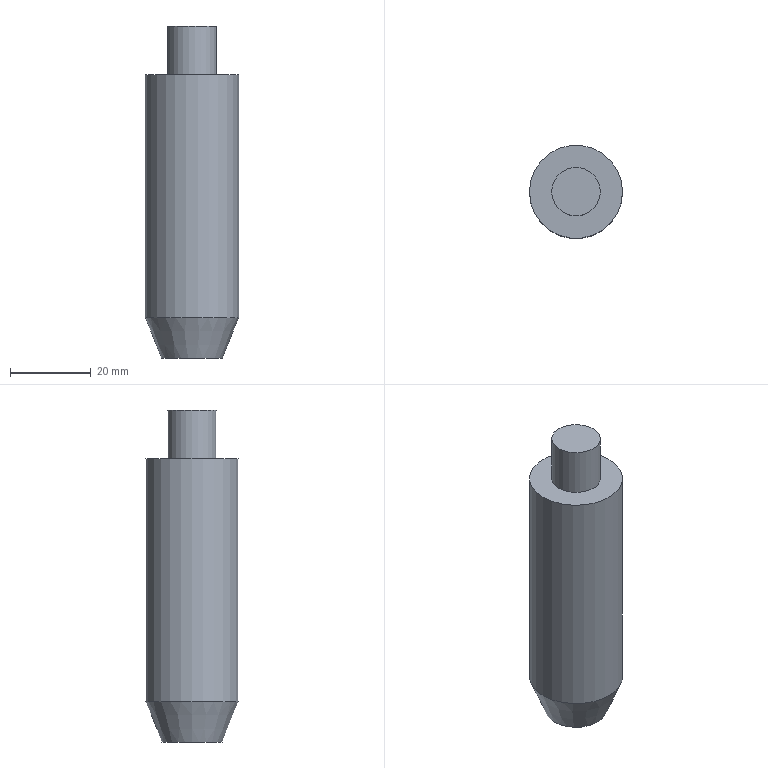Part | NX | features solid 2 | 1 solid | 6 faces | box 23 x 23 x 82 mm | volume 29163 mm3 | plane 3 | cylinder 2 | cone 1 | commonest cylinder face diameters 12 x1 23 x1
STEP:
#1=CARTESIAN_POINT('',(941.784,-40.121,180.));
#2=VERTEX_POINT('',#1);
#3=CARTESIAN_POINT('',(953.284,-40.121,180.));
#4=DIRECTION('',(0.,0.,-1.));
#5=DIRECTION('',(-1.,0.,0.));
#6=AXIS2_PLACEMENT_3D('',#3,#4,#5);
#7=CIRCLE('',#6,11.5);
#8=EDGE_CURVE('',#2,#2,#7,.T.);
#9=ORIENTED_EDGE('',*,*,#8,.F.);
#10=EDGE_LOOP('',(#9));
#11=FACE_BOUND('',#10,.T.);
#12=CARTESIAN_POINT('',(941.784,-40.121,240.));
#13=VERTEX_POINT('',#12);
#14=CARTESIAN_POINT('',(953.284,-40.121,240.));
#15=DIRECTION('',(0.,0.,-1.));
#16=DIRECTION('',(-1.,0.,0.));
#17=AXIS2_PLACEMENT_3D('',#14,#15,#16);
#18=CIRCLE('',#17,11.5);
#19=EDGE_CURVE('',#13,#13,#18,.T.);
#20=ORIENTED_EDGE('',*,*,#19,.T.);
#21=EDGE_LOOP('',(#20));
#22=FACE_BOUND('',#21,.T.);
#23=CARTESIAN_POINT('',(953.284,-40.121,240.));
#24=DIRECTION('',(0.,0.,-1.));
#25=DIRECTION('',(1.,0.,0.));
#26=AXIS2_PLACEMENT_3D('',#23,#24,#25);
#27=CYLINDRICAL_SURFACE('',#26,11.5);
#28=ADVANCED_FACE('',(#11,#22),#27,.T.);
#29=CARTESIAN_POINT('',(947.284,-40.121,240.));
#30=VERTEX_POINT('',#29);
#31=CARTESIAN_POINT('',(953.284,-40.121,240.));
#32=DIRECTION('',(0.,0.,-1.));
#33=DIRECTION('',(-1.,0.,0.));
#34=AXIS2_PLACEMENT_3D('',#31,#32,#33);
#35=CIRCLE('',#34,6.);
#36=EDGE_CURVE('',#30,#30,#35,.T.);
#37=ORIENTED_EDGE('',*,*,#36,.T.);
#38=EDGE_LOOP('',(#37));
#39=FACE_BOUND('',#38,.T.);
#40=ORIENTED_EDGE('',*,*,#19,.F.);
#41=EDGE_LOOP('',(#40));
#42=FACE_BOUND('',#41,.T.);
#43=CARTESIAN_POINT('',(953.284,-40.121,240.));
#44=DIRECTION('',(0.,0.,1.));
#45=DIRECTION('',(-1.,0.,0.));
#46=AXIS2_PLACEMENT_3D('',#43,#44,#45);
#47=PLANE('',#46);
#48=ADVANCED_FACE('',(#39,#42),#47,.T.);
#49=CARTESIAN_POINT('',(945.784,-40.121,170.));
#50=VERTEX_POINT('',#49);
#51=CARTESIAN_POINT('',(953.284,-40.121,170.));
#52=DIRECTION('',(0.,0.,-1.));
#53=DIRECTION('',(-1.,0.,0.));
#54=AXIS2_PLACEMENT_3D('',#51,#52,#53);
#55=CIRCLE('',#54,7.5);
#56=EDGE_CURVE('',#50,#50,#55,.F.);
#57=ORIENTED_EDGE('',*,*,#56,.F.);
#58=EDGE_LOOP('',(#57));
#59=FACE_BOUND('',#58,.T.);
#60=CARTESIAN_POINT('',(953.284,-40.121,170.));
#61=DIRECTION('',(0.,0.,1.));
#62=DIRECTION('',(-1.,0.,0.));
#63=AXIS2_PLACEMENT_3D('',#60,#61,#62);
#64=PLANE('',#63);
#65=ADVANCED_FACE('',(#59),#64,.F.);
#66=ORIENTED_EDGE('',*,*,#36,.F.);
#67=EDGE_LOOP('',(#66));
#68=FACE_BOUND('',#67,.T.);
#69=CARTESIAN_POINT('',(947.284,-40.121,252.));
#70=VERTEX_POINT('',#69);
#71=CARTESIAN_POINT('',(953.284,-40.121,252.));
#72=DIRECTION('',(0.,0.,-1.));
#73=DIRECTION('',(-1.,0.,0.));
#74=AXIS2_PLACEMENT_3D('',#71,#72,#73);
#75=CIRCLE('',#74,6.);
#76=EDGE_CURVE('',#70,#70,#75,.T.);
#77=ORIENTED_EDGE('',*,*,#76,.T.);
#78=EDGE_LOOP('',(#77));
#79=FACE_BOUND('',#78,.T.);
#80=CARTESIAN_POINT('',(953.284,-40.121,240.));
#81=DIRECTION('',(0.,0.,1.));
#82=DIRECTION('',(-1.,0.,0.));
#83=AXIS2_PLACEMENT_3D('',#80,#81,#82);
#84=CYLINDRICAL_SURFACE('',#83,6.);
#85=ADVANCED_FACE('',(#68,#79),#84,.T.);
#86=ORIENTED_EDGE('',*,*,#76,.F.);
#87=EDGE_LOOP('',(#86));
#88=FACE_BOUND('',#87,.T.);
#89=CARTESIAN_POINT('',(953.284,-40.121,252.));
#90=DIRECTION('',(0.,0.,1.));
#91=DIRECTION('',(-1.,0.,0.));
#92=AXIS2_PLACEMENT_3D('',#89,#90,#91);
#93=PLANE('',#92);
#94=ADVANCED_FACE('',(#88),#93,.T.);
#95=ORIENTED_EDGE('',*,*,#56,.T.);
#96=EDGE_LOOP('',(#95));
#97=FACE_BOUND('',#96,.T.);
#98=ORIENTED_EDGE('',*,*,#8,.T.);
#99=EDGE_LOOP('',(#98));
#100=FACE_BOUND('',#99,.T.);
#101=CARTESIAN_POINT('',(953.284,-40.121,180.));
#102=DIRECTION('',(0.,0.,1.));
#103=DIRECTION('',(-1.,0.,0.));
#104=AXIS2_PLACEMENT_3D('',#101,#102,#103);
#105=CONICAL_SURFACE('',#104,11.5,0.3805);
#106=ADVANCED_FACE('',(#97,#100),#105,.T.);
#107=CLOSED_SHELL('',(#28,#48,#65,#85,#94,#106));
#108=MANIFOLD_SOLID_BREP('',#107);
#109=(LENGTH_UNIT()NAMED_UNIT(*)SI_UNIT(.MILLI.,.METRE.));
#110=UNCERTAINTY_MEASURE_WITH_UNIT(LENGTH_MEASURE(0.00001),#109,'','');
#111=(NAMED_UNIT(*)PLANE_ANGLE_UNIT()SI_UNIT($,.RADIAN.));
#112=(NAMED_UNIT(*)SI_UNIT($,.STERADIAN.)SOLID_ANGLE_UNIT());
#113=(GEOMETRIC_REPRESENTATION_CONTEXT(3)GLOBAL_UNCERTAINTY_ASSIGNED_CONTEXT((#110))GLOBAL_UNIT_ASSIGNED_CONTEXT((#109,#111,#112))REPRESENTATION_CONTEXT('',''));
#114=ADVANCED_BREP_SHAPE_REPRESENTATION('',(#108),#113);